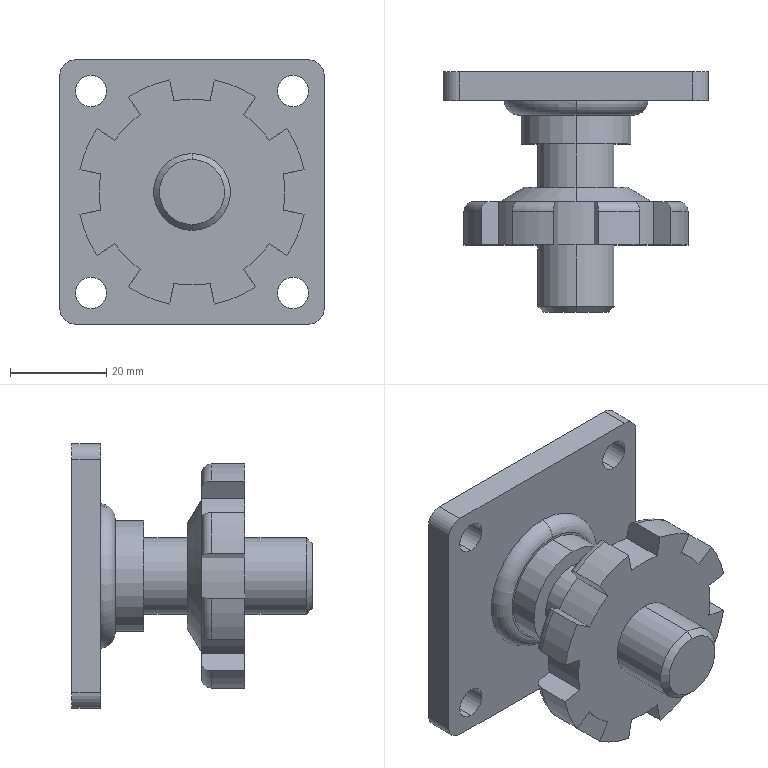Part | NX | features BREP 1 | 1 solid | 101 faces | box 55 x 50 x 55 mm | volume 38806 mm3 | plane 45 | cylinder 42 | torus 10 | cone 4 | commonest cylinder face diameters 6.5 x12 38.667 x9 47.5 x8 16 x6 10.667 x5 23 x2